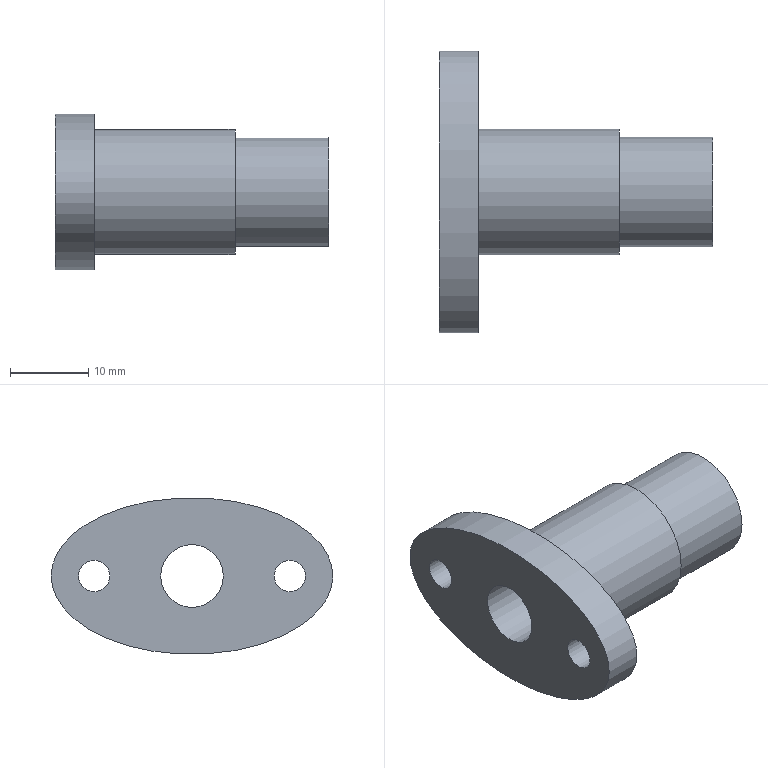Part | STEP file | 1-56.14 | 1 solid | 11 faces | box 35 x 36 x 20 mm | volume 6413 mm3 | cylinder 6 | plane 4 | spline 1 | commonest cylinder face diameters 4 x2 8 x2 14 x1 16 x1
STEP:
#1=CARTESIAN_POINT('',(0.,0.,0.));
#2=DIRECTION('',(0.,0.,1.));
#3=DIRECTION('',(1.,0.,0.));
#4=AXIS2_PLACEMENT_3D('',#1,#2,#3);
#5=CARTESIAN_POINT('',(-5.,18.,0.));
#6=VERTEX_POINT('',#5);
#7=CARTESIAN_POINT('',(-5.,0.,0.));
#8=DIRECTION('',(1.,0.,0.));
#9=DIRECTION('',(0.,1.,0.));
#10=AXIS2_PLACEMENT_3D('',#7,#8,#9);
#11=ELLIPSE('',#10,18.,10.);
#12=CARTESIAN_POINT('',(-5.,0.,-8.));
#13=DIRECTION('',(1.,0.,0.));
#14=DIRECTION('',(0.,0.,-1.));
#15=AXIS2_PLACEMENT_3D('',#12,#13,#14);
#16=PLANE('',#15);
#17=CARTESIAN_POINT('',(-8.,0.));
#18=DIRECTION('',(0.,1.));
#19=AXIS2_PLACEMENT_2D('',#17,#18);
#20=ELLIPSE('',#19,18.,10.);
#21=(GEOMETRIC_REPRESENTATION_CONTEXT(2)PARAMETRIC_REPRESENTATION_CONTEXT()REPRESENTATION_CONTEXT('',''));
#22=DEFINITIONAL_REPRESENTATION('',(#20),#21);
#23=PCURVE('',#16,#22);
#24=CARTESIAN_POINT('',(0.,18.,0.));
#25=CARTESIAN_POINT('',(-5.,18.,0.));
#26=CARTESIAN_POINT('',(0.,18.,10.));
#27=CARTESIAN_POINT('',(-5.,18.,10.));
#28=CARTESIAN_POINT('',(0.,0.,10.));
#29=CARTESIAN_POINT('',(-5.,0.,10.));
#30=CARTESIAN_POINT('',(0.,-18.,10.));
#31=CARTESIAN_POINT('',(-5.,-18.,10.));
#32=CARTESIAN_POINT('',(0.,-18.,0.));
#33=CARTESIAN_POINT('',(-5.,-18.,0.));
#34=CARTESIAN_POINT('',(0.,-18.,-10.));
#35=CARTESIAN_POINT('',(-5.,-18.,-10.));
#36=CARTESIAN_POINT('',(0.,0.,-10.));
#37=CARTESIAN_POINT('',(-5.,0.,-10.));
#38=CARTESIAN_POINT('',(0.,18.,-10.));
#39=CARTESIAN_POINT('',(-5.,18.,-10.));
#40=CARTESIAN_POINT('',(0.,18.,0.));
#41=CARTESIAN_POINT('',(-5.,18.,0.));
#42=(BOUNDED_SURFACE()B_SPLINE_SURFACE(2,1,((#24,#25),(#26,#27),(#28,#29),(#30,#31),(#32,#33),(#34,#35),(#36,#37),(#38,#39),(#40,#41)),.UNSPECIFIED.,.T.,.F.,.F.)B_SPLINE_SURFACE_WITH_KNOTS((1,2,2,2,2,2,1),(2,2),(-0.25,0.,0.25,0.5,0.75,1.,1.25),(0.,1.),.UNSPECIFIED.)GEOMETRIC_REPRESENTATION_ITEM()RATIONAL_B_SPLINE_SURFACE(((1.,1.),(0.7071,0.7071),(1.,1.),(0.7071,0.7071),(1.,1.),(0.7071,0.7071),(1.,1.),(0.7071,0.7071),(1.,1.)))REPRESENTATION_ITEM('')SURFACE());
#43=CARTESIAN_POINT('',(0.,1.));
#44=CARTESIAN_POINT('',(0.01678,1.));
#45=CARTESIAN_POINT('',(0.04854,1.));
#46=CARTESIAN_POINT('',(0.09277,1.));
#47=CARTESIAN_POINT('',(0.1357,1.));
#48=CARTESIAN_POINT('',(0.1791,1.));
#49=CARTESIAN_POINT('',(0.2245,1.));
#50=CARTESIAN_POINT('',(0.2755,1.));
#51=CARTESIAN_POINT('',(0.3209,1.));
#52=CARTESIAN_POINT('',(0.3643,1.));
#53=CARTESIAN_POINT('',(0.4073,1.));
#54=CARTESIAN_POINT('',(0.4512,1.));
#55=CARTESIAN_POINT('',(0.5,1.));
#56=CARTESIAN_POINT('',(0.5488,1.));
#57=CARTESIAN_POINT('',(0.5927,1.));
#58=CARTESIAN_POINT('',(0.6357,1.));
#59=CARTESIAN_POINT('',(0.6791,1.));
#60=CARTESIAN_POINT('',(0.7245,1.));
#61=CARTESIAN_POINT('',(0.7755,1.));
#62=CARTESIAN_POINT('',(0.8209,1.));
#63=CARTESIAN_POINT('',(0.8643,1.));
#64=CARTESIAN_POINT('',(0.9072,1.));
#65=CARTESIAN_POINT('',(0.9515,1.));
#66=CARTESIAN_POINT('',(0.9832,1.));
#67=CARTESIAN_POINT('',(1.,1.));
#68=B_SPLINE_CURVE_WITH_KNOTS('',3,(#43,#44,#45,#46,#47,#48,#49,#50,#51,#52,#53,#54,#55,#56,#57,#58,#59,#60,#61,#62,#63,#64,#65,#66,#67),.UNSPECIFIED.,.F.,.F.,(4,1,1,1,1,1,1,1,1,1,1,1,1,1,1,1,1,1,1,1,1,1,4),(0.,0.2856,0.5712,0.8568,1.142,1.428,1.714,1.999,2.285,2.57,2.856,3.142,3.427,3.713,3.998,4.284,4.57,4.855,5.141,5.426,5.712,5.998,6.283),.QUASI_UNIFORM_KNOTS.);
#69=(GEOMETRIC_REPRESENTATION_CONTEXT(2)PARAMETRIC_REPRESENTATION_CONTEXT()REPRESENTATION_CONTEXT('',''));
#70=DEFINITIONAL_REPRESENTATION('',(#68),#69);
#71=PCURVE('',#42,#70);
#72=SURFACE_CURVE('',#11,(#23,#71),.PCURVE_S1.);
#73=EDGE_CURVE('',#6,#6,#72,.T.);
#74=ORIENTED_EDGE('',*,*,#73,.T.);
#75=EDGE_LOOP('',(#74));
#76=FACE_BOUND('',#75,.F.);
#77=CARTESIAN_POINT('',(-5.,14.5,0.));
#78=VERTEX_POINT('',#77);
#79=CARTESIAN_POINT('',(-5.,12.5,0.));
#80=DIRECTION('',(-1.,0.,0.));
#81=DIRECTION('',(0.,1.,0.));
#82=AXIS2_PLACEMENT_3D('',#79,#80,#81);
#83=CIRCLE('',#82,2.);
#84=CARTESIAN_POINT('',(-8.,14.5));
#85=CARTESIAN_POINT('',(-4.536,14.5));
#86=CARTESIAN_POINT('',(-6.268,11.5));
#87=CARTESIAN_POINT('',(-8.,8.5));
#88=CARTESIAN_POINT('',(-9.732,11.5));
#89=CARTESIAN_POINT('',(-11.464,14.5));
#90=CARTESIAN_POINT('',(-8.,14.5));
#91=(BOUNDED_CURVE()B_SPLINE_CURVE(2,(#84,#85,#86,#87,#88,#89,#90),.UNSPECIFIED.,.T.,.F.)B_SPLINE_CURVE_WITH_KNOTS((1,2,2,2,2,1),(-2.094,0.,2.094,4.189,6.283,8.378),.UNSPECIFIED.)CURVE()GEOMETRIC_REPRESENTATION_ITEM()RATIONAL_B_SPLINE_CURVE((1.,0.5,1.,0.5,1.,0.5,1.))REPRESENTATION_ITEM(''));
#92=(GEOMETRIC_REPRESENTATION_CONTEXT(2)PARAMETRIC_REPRESENTATION_CONTEXT()REPRESENTATION_CONTEXT('',''));
#93=DEFINITIONAL_REPRESENTATION('',(#91),#92);
#94=PCURVE('',#16,#93);
#95=CARTESIAN_POINT('',(0.,12.5,0.));
#96=DIRECTION('',(-1.,0.,0.));
#97=DIRECTION('',(0.,1.,0.));
#98=AXIS2_PLACEMENT_3D('',#95,#96,#97);
#99=CYLINDRICAL_SURFACE('',#98,2.);
#100=CARTESIAN_POINT('',(0.,5.));
#101=DIRECTION('',(1.,0.));
#102=VECTOR('',#101,1.);
#103=LINE('',#100,#102);
#104=(GEOMETRIC_REPRESENTATION_CONTEXT(2)PARAMETRIC_REPRESENTATION_CONTEXT()REPRESENTATION_CONTEXT('',''));
#105=DEFINITIONAL_REPRESENTATION('',(#103),#104);
#106=PCURVE('',#99,#105);
#107=SURFACE_CURVE('',#83,(#94,#106),.PCURVE_S1.);
#108=EDGE_CURVE('',#78,#78,#107,.T.);
#109=ORIENTED_EDGE('',*,*,#108,.T.);
#110=EDGE_LOOP('',(#109));
#111=FACE_BOUND('',#110,.F.);
#112=CARTESIAN_POINT('',(-5.,-10.5,0.));
#113=VERTEX_POINT('',#112);
#114=CARTESIAN_POINT('',(-5.,-12.5,0.));
#115=DIRECTION('',(-1.,0.,0.));
#116=DIRECTION('',(0.,1.,0.));
#117=AXIS2_PLACEMENT_3D('',#114,#115,#116);
#118=CIRCLE('',#117,2.);
#119=CARTESIAN_POINT('',(-8.,-10.5));
#120=CARTESIAN_POINT('',(-4.536,-10.5));
#121=CARTESIAN_POINT('',(-6.268,-13.5));
#122=CARTESIAN_POINT('',(-8.,-16.5));
#123=CARTESIAN_POINT('',(-9.732,-13.5));
#124=CARTESIAN_POINT('',(-11.464,-10.5));
#125=CARTESIAN_POINT('',(-8.,-10.5));
#126=(BOUNDED_CURVE()B_SPLINE_CURVE(2,(#119,#120,#121,#122,#123,#124,#125),.UNSPECIFIED.,.T.,.F.)B_SPLINE_CURVE_WITH_KNOTS((1,2,2,2,2,1),(-2.094,0.,2.094,4.189,6.283,8.378),.UNSPECIFIED.)CURVE()GEOMETRIC_REPRESENTATION_ITEM()RATIONAL_B_SPLINE_CURVE((1.,0.5,1.,0.5,1.,0.5,1.))REPRESENTATION_ITEM(''));
#127=(GEOMETRIC_REPRESENTATION_CONTEXT(2)PARAMETRIC_REPRESENTATION_CONTEXT()REPRESENTATION_CONTEXT('',''));
#128=DEFINITIONAL_REPRESENTATION('',(#126),#127);
#129=PCURVE('',#16,#128);
#130=CARTESIAN_POINT('',(0.,-12.5,0.));
#131=DIRECTION('',(-1.,0.,0.));
#132=DIRECTION('',(0.,1.,0.));
#133=AXIS2_PLACEMENT_3D('',#130,#131,#132);
#134=CYLINDRICAL_SURFACE('',#133,2.);
#135=CARTESIAN_POINT('',(0.,5.));
#136=DIRECTION('',(1.,0.));
#137=VECTOR('',#136,1.);
#138=LINE('',#135,#137);
#139=(GEOMETRIC_REPRESENTATION_CONTEXT(2)PARAMETRIC_REPRESENTATION_CONTEXT()REPRESENTATION_CONTEXT('',''));
#140=DEFINITIONAL_REPRESENTATION('',(#138),#139);
#141=PCURVE('',#134,#140);
#142=SURFACE_CURVE('',#118,(#129,#141),.PCURVE_S1.);
#143=EDGE_CURVE('',#113,#113,#142,.T.);
#144=ORIENTED_EDGE('',*,*,#143,.T.);
#145=EDGE_LOOP('',(#144));
#146=FACE_BOUND('',#145,.F.);
#147=CARTESIAN_POINT('',(-5.,4.,0.));
#148=VERTEX_POINT('',#147);
#149=CARTESIAN_POINT('',(-5.,0.,0.));
#150=DIRECTION('',(-1.,0.,0.));
#151=DIRECTION('',(0.,1.,0.));
#152=AXIS2_PLACEMENT_3D('',#149,#150,#151);
#153=CIRCLE('',#152,4.);
#154=CARTESIAN_POINT('',(-8.,4.));
#155=CARTESIAN_POINT('',(-1.072,4.));
#156=CARTESIAN_POINT('',(-4.536,-2.));
#157=CARTESIAN_POINT('',(-8.,-8.));
#158=CARTESIAN_POINT('',(-11.464,-2.));
#159=CARTESIAN_POINT('',(-14.928,4.));
#160=CARTESIAN_POINT('',(-8.,4.));
#161=(BOUNDED_CURVE()B_SPLINE_CURVE(2,(#154,#155,#156,#157,#158,#159,#160),.UNSPECIFIED.,.T.,.F.)B_SPLINE_CURVE_WITH_KNOTS((1,2,2,2,2,1),(-2.094,0.,2.094,4.189,6.283,8.378),.UNSPECIFIED.)CURVE()GEOMETRIC_REPRESENTATION_ITEM()RATIONAL_B_SPLINE_CURVE((1.,0.5,1.,0.5,1.,0.5,1.))REPRESENTATION_ITEM(''));
#162=(GEOMETRIC_REPRESENTATION_CONTEXT(2)PARAMETRIC_REPRESENTATION_CONTEXT()REPRESENTATION_CONTEXT('',''));
#163=DEFINITIONAL_REPRESENTATION('',(#161),#162);
#164=PCURVE('',#16,#163);
#165=CARTESIAN_POINT('',(30.,0.,0.));
#166=DIRECTION('',(-1.,0.,0.));
#167=DIRECTION('',(0.,1.,0.));
#168=AXIS2_PLACEMENT_3D('',#165,#166,#167);
#169=CYLINDRICAL_SURFACE('',#168,4.);
#170=CARTESIAN_POINT('',(0.,35.));
#171=DIRECTION('',(1.,0.));
#172=VECTOR('',#171,1.);
#173=LINE('',#170,#172);
#174=(GEOMETRIC_REPRESENTATION_CONTEXT(2)PARAMETRIC_REPRESENTATION_CONTEXT()REPRESENTATION_CONTEXT('',''));
#175=DEFINITIONAL_REPRESENTATION('',(#173),#174);
#176=PCURVE('',#169,#175);
#177=SURFACE_CURVE('',#153,(#164,#176),.PCURVE_S1.);
#178=EDGE_CURVE('',#148,#148,#177,.T.);
#179=ORIENTED_EDGE('',*,*,#178,.T.);
#180=EDGE_LOOP('',(#179));
#181=FACE_BOUND('',#180,.F.);
#182=ADVANCED_FACE('',(#76,#111,#146,#181),#16,.F.);
#183=CARTESIAN_POINT('',(0.,18.,0.));
#184=VERTEX_POINT('',#183);
#185=CARTESIAN_POINT('',(0.,0.,0.));
#186=DIRECTION('',(1.,0.,0.));
#187=DIRECTION('',(0.,1.,0.));
#188=AXIS2_PLACEMENT_3D('',#185,#186,#187);
#189=ELLIPSE('',#188,18.,10.);
#190=CARTESIAN_POINT('',(0.,0.));
#191=CARTESIAN_POINT('',(0.01678,0.));
#192=CARTESIAN_POINT('',(0.04854,0.));
#193=CARTESIAN_POINT('',(0.09277,0.));
#194=CARTESIAN_POINT('',(0.1357,0.));
#195=CARTESIAN_POINT('',(0.1791,0.));
#196=CARTESIAN_POINT('',(0.2245,0.));
#197=CARTESIAN_POINT('',(0.2755,0.));
#198=CARTESIAN_POINT('',(0.3209,0.));
#199=CARTESIAN_POINT('',(0.3643,0.));
#200=CARTESIAN_POINT('',(0.4073,0.));
#201=CARTESIAN_POINT('',(0.4512,0.));
#202=CARTESIAN_POINT('',(0.5,0.));
#203=CARTESIAN_POINT('',(0.5488,0.));
#204=CARTESIAN_POINT('',(0.5927,0.));
#205=CARTESIAN_POINT('',(0.6357,0.));
#206=CARTESIAN_POINT('',(0.6791,0.));
#207=CARTESIAN_POINT('',(0.7245,0.));
#208=CARTESIAN_POINT('',(0.7755,0.));
#209=CARTESIAN_POINT('',(0.8209,0.));
#210=CARTESIAN_POINT('',(0.8643,0.));
#211=CARTESIAN_POINT('',(0.9072,0.));
#212=CARTESIAN_POINT('',(0.9515,0.));
#213=CARTESIAN_POINT('',(0.9832,0.));
#214=CARTESIAN_POINT('',(1.,0.));
#215=B_SPLINE_CURVE_WITH_KNOTS('',3,(#190,#191,#192,#193,#194,#195,#196,#197,#198,#199,#200,#201,#202,#203,#204,#205,#206,#207,#208,#209,#210,#211,#212,#213,#214),.UNSPECIFIED.,.F.,.F.,(4,1,1,1,1,1,1,1,1,1,1,1,1,1,1,1,1,1,1,1,1,1,4),(0.,0.2856,0.5712,0.8568,1.142,1.428,1.714,1.999,2.285,2.57,2.856,3.142,3.427,3.713,3.998,4.284,4.57,4.855,5.141,5.426,5.712,5.998,6.283),.QUASI_UNIFORM_KNOTS.);
#216=(GEOMETRIC_REPRESENTATION_CONTEXT(2)PARAMETRIC_REPRESENTATION_CONTEXT()REPRESENTATION_CONTEXT('',''));
#217=DEFINITIONAL_REPRESENTATION('',(#215),#216);
#218=PCURVE('',#42,#217);
#219=CARTESIAN_POINT('',(0.,0.,-8.));
#220=DIRECTION('',(1.,0.,0.));
#221=DIRECTION('',(0.,0.,-1.));
#222=AXIS2_PLACEMENT_3D('',#219,#220,#221);
#223=PLANE('',#222);
#224=CARTESIAN_POINT('',(-8.,0.));
#225=DIRECTION('',(0.,1.));
#226=AXIS2_PLACEMENT_2D('',#224,#225);
#227=ELLIPSE('',#226,18.,10.);
#228=(GEOMETRIC_REPRESENTATION_CONTEXT(2)PARAMETRIC_REPRESENTATION_CONTEXT()REPRESENTATION_CONTEXT('',''));
#229=DEFINITIONAL_REPRESENTATION('',(#227),#228);
#230=PCURVE('',#223,#229);
#231=SURFACE_CURVE('',#189,(#218,#230),.PCURVE_S1.);
#232=EDGE_CURVE('',#184,#184,#231,.T.);
#233=ORIENTED_EDGE('',*,*,#232,.T.);
#234=CARTESIAN_POINT('',(0.,18.,0.));
#235=DIRECTION('',(-1.,0.,0.));
#236=VECTOR('',#235,1.);
#237=LINE('',#234,#236);
#238=CARTESIAN_POINT('',(1.,0.));
#239=CARTESIAN_POINT('',(1.,1.));
#240=B_SPLINE_CURVE_WITH_KNOTS('',1,(#238,#239),.UNSPECIFIED.,.F.,.F.,(2,2),(0.,5.),.PIECEWISE_BEZIER_KNOTS.);
#241=(GEOMETRIC_REPRESENTATION_CONTEXT(2)PARAMETRIC_REPRESENTATION_CONTEXT()REPRESENTATION_CONTEXT('',''));
#242=DEFINITIONAL_REPRESENTATION('',(#240),#241);
#243=PCURVE('',#42,#242);
#244=CARTESIAN_POINT('',(0.,0.));
#245=CARTESIAN_POINT('',(0.,1.));
#246=B_SPLINE_CURVE_WITH_KNOTS('',1,(#244,#245),.UNSPECIFIED.,.F.,.F.,(2,2),(0.,5.),.PIECEWISE_BEZIER_KNOTS.);
#247=(GEOMETRIC_REPRESENTATION_CONTEXT(2)PARAMETRIC_REPRESENTATION_CONTEXT()REPRESENTATION_CONTEXT('',''));
#248=DEFINITIONAL_REPRESENTATION('',(#246),#247);
#249=PCURVE('',#42,#248);
#250=SEAM_CURVE('',#237,(#243,#249),.PCURVE_S1.);
#251=EDGE_CURVE('',#184,#6,#250,.T.);
#252=ORIENTED_EDGE('',*,*,#251,.T.);
#253=ORIENTED_EDGE('',*,*,#73,.F.);
#254=ORIENTED_EDGE('',*,*,#251,.F.);
#255=EDGE_LOOP('',(#233,#252,#253,#254));
#256=FACE_BOUND('',#255,.F.);
#257=ADVANCED_FACE('',(#256),#42,.F.);
#258=CARTESIAN_POINT('',(0.,14.5,0.));
#259=VERTEX_POINT('',#258);
#260=CARTESIAN_POINT('',(0.,12.5,0.));
#261=DIRECTION('',(-1.,0.,0.));
#262=DIRECTION('',(0.,1.,0.));
#263=AXIS2_PLACEMENT_3D('',#260,#261,#262);
#264=CIRCLE('',#263,2.);
#265=CARTESIAN_POINT('',(0.,0.));
#266=DIRECTION('',(1.,0.));
#267=VECTOR('',#266,1.);
#268=LINE('',#265,#267);
#269=(GEOMETRIC_REPRESENTATION_CONTEXT(2)PARAMETRIC_REPRESENTATION_CONTEXT()REPRESENTATION_CONTEXT('',''));
#270=DEFINITIONAL_REPRESENTATION('',(#268),#269);
#271=PCURVE('',#99,#270);
#272=CARTESIAN_POINT('',(-8.,14.5));
#273=CARTESIAN_POINT('',(-4.536,14.5));
#274=CARTESIAN_POINT('',(-6.268,11.5));
#275=CARTESIAN_POINT('',(-8.,8.5));
#276=CARTESIAN_POINT('',(-9.732,11.5));
#277=CARTESIAN_POINT('',(-11.464,14.5));
#278=CARTESIAN_POINT('',(-8.,14.5));
#279=(BOUNDED_CURVE()B_SPLINE_CURVE(2,(#272,#273,#274,#275,#276,#277,#278),.UNSPECIFIED.,.T.,.F.)B_SPLINE_CURVE_WITH_KNOTS((1,2,2,2,2,1),(-2.094,0.,2.094,4.189,6.283,8.378),.UNSPECIFIED.)CURVE()GEOMETRIC_REPRESENTATION_ITEM()RATIONAL_B_SPLINE_CURVE((1.,0.5,1.,0.5,1.,0.5,1.))REPRESENTATION_ITEM(''));
#280=(GEOMETRIC_REPRESENTATION_CONTEXT(2)PARAMETRIC_REPRESENTATION_CONTEXT()REPRESENTATION_CONTEXT('',''));
#281=DEFINITIONAL_REPRESENTATION('',(#279),#280);
#282=PCURVE('',#223,#281);
#283=SURFACE_CURVE('',#264,(#271,#282),.PCURVE_S1.);
#284=EDGE_CURVE('',#259,#259,#283,.T.);
#285=ORIENTED_EDGE('',*,*,#284,.T.);
#286=CARTESIAN_POINT('',(0.,14.5,0.));
#287=DIRECTION('',(-1.,0.,0.));
#288=VECTOR('',#287,1.);
#289=LINE('',#286,#288);
#290=CARTESIAN_POINT('',(6.283,0.));
#291=DIRECTION('',(0.,1.));
#292=VECTOR('',#291,1.);
#293=LINE('',#290,#292);
#294=(GEOMETRIC_REPRESENTATION_CONTEXT(2)PARAMETRIC_REPRESENTATION_CONTEXT()REPRESENTATION_CONTEXT('',''));
#295=DEFINITIONAL_REPRESENTATION('',(#293),#294);
#296=PCURVE('',#99,#295);
#297=CARTESIAN_POINT('',(0.,0.));
#298=DIRECTION('',(0.,1.));
#299=VECTOR('',#298,1.);
#300=LINE('',#297,#299);
#301=(GEOMETRIC_REPRESENTATION_CONTEXT(2)PARAMETRIC_REPRESENTATION_CONTEXT()REPRESENTATION_CONTEXT('',''));
#302=DEFINITIONAL_REPRESENTATION('',(#300),#301);
#303=PCURVE('',#99,#302);
#304=SEAM_CURVE('',#289,(#296,#303),.PCURVE_S1.);
#305=EDGE_CURVE('',#259,#78,#304,.T.);
#306=ORIENTED_EDGE('',*,*,#305,.T.);
#307=ORIENTED_EDGE('',*,*,#108,.F.);
#308=ORIENTED_EDGE('',*,*,#305,.F.);
#309=EDGE_LOOP('',(#285,#306,#307,#308));
#310=FACE_BOUND('',#309,.F.);
#311=ADVANCED_FACE('',(#310),#99,.F.);
#312=CARTESIAN_POINT('',(0.,-10.5,0.));
#313=VERTEX_POINT('',#312);
#314=CARTESIAN_POINT('',(0.,-12.5,0.));
#315=DIRECTION('',(-1.,0.,0.));
#316=DIRECTION('',(0.,1.,0.));
#317=AXIS2_PLACEMENT_3D('',#314,#315,#316);
#318=CIRCLE('',#317,2.);
#319=CARTESIAN_POINT('',(0.,0.));
#320=DIRECTION('',(1.,0.));
#321=VECTOR('',#320,1.);
#322=LINE('',#319,#321);
#323=(GEOMETRIC_REPRESENTATION_CONTEXT(2)PARAMETRIC_REPRESENTATION_CONTEXT()REPRESENTATION_CONTEXT('',''));
#324=DEFINITIONAL_REPRESENTATION('',(#322),#323);
#325=PCURVE('',#134,#324);
#326=CARTESIAN_POINT('',(-8.,-10.5));
#327=CARTESIAN_POINT('',(-4.536,-10.5));
#328=CARTESIAN_POINT('',(-6.268,-13.5));
#329=CARTESIAN_POINT('',(-8.,-16.5));
#330=CARTESIAN_POINT('',(-9.732,-13.5));
#331=CARTESIAN_POINT('',(-11.464,-10.5));
#332=CARTESIAN_POINT('',(-8.,-10.5));
#333=(BOUNDED_CURVE()B_SPLINE_CURVE(2,(#326,#327,#328,#329,#330,#331,#332),.UNSPECIFIED.,.T.,.F.)B_SPLINE_CURVE_WITH_KNOTS((1,2,2,2,2,1),(-2.094,0.,2.094,4.189,6.283,8.378),.UNSPECIFIED.)CURVE()GEOMETRIC_REPRESENTATION_ITEM()RATIONAL_B_SPLINE_CURVE((1.,0.5,1.,0.5,1.,0.5,1.))REPRESENTATION_ITEM(''));
#334=(GEOMETRIC_REPRESENTATION_CONTEXT(2)PARAMETRIC_REPRESENTATION_CONTEXT()REPRESENTATION_CONTEXT('',''));
#335=DEFINITIONAL_REPRESENTATION('',(#333),#334);
#336=PCURVE('',#223,#335);
#337=SURFACE_CURVE('',#318,(#325,#336),.PCURVE_S1.);
#338=EDGE_CURVE('',#313,#313,#337,.T.);
#339=ORIENTED_EDGE('',*,*,#338,.T.);
#340=CARTESIAN_POINT('',(0.,-10.5,0.));
#341=DIRECTION('',(-1.,0.,0.));
#342=VECTOR('',#341,1.);
#343=LINE('',#340,#342);
#344=CARTESIAN_POINT('',(6.283,0.));
#345=DIRECTION('',(0.,1.));
#346=VECTOR('',#345,1.);
#347=LINE('',#344,#346);
#348=(GEOMETRIC_REPRESENTATION_CONTEXT(2)PARAMETRIC_REPRESENTATION_CONTEXT()REPRESENTATION_CONTEXT('',''));
#349=DEFINITIONAL_REPRESENTATION('',(#347),#348);
#350=PCURVE('',#134,#349);
#351=CARTESIAN_POINT('',(0.,0.));
#352=DIRECTION('',(0.,1.));
#353=VECTOR('',#352,1.);
#354=LINE('',#351,#353);
#355=(GEOMETRIC_REPRESENTATION_CONTEXT(2)PARAMETRIC_REPRESENTATION_CONTEXT()REPRESENTATION_CONTEXT('',''));
#356=DEFINITIONAL_REPRESENTATION('',(#354),#355);
#357=PCURVE('',#134,#356);
#358=SEAM_CURVE('',#343,(#350,#357),.PCURVE_S1.);
#359=EDGE_CURVE('',#313,#113,#358,.T.);
#360=ORIENTED_EDGE('',*,*,#359,.T.);
#361=ORIENTED_EDGE('',*,*,#143,.F.);
#362=ORIENTED_EDGE('',*,*,#359,.F.);
#363=EDGE_LOOP('',(#339,#360,#361,#362));
#364=FACE_BOUND('',#363,.F.);
#365=ADVANCED_FACE('',(#364),#134,.F.);
#366=ORIENTED_EDGE('',*,*,#232,.T.);
#367=EDGE_LOOP('',(#366));
#368=FACE_BOUND('',#367,.T.);
#369=CARTESIAN_POINT('',(0.,8.,0.));
#370=VERTEX_POINT('',#369);
#371=CARTESIAN_POINT('',(0.,0.,0.));
#372=DIRECTION('',(1.,0.,0.));
#373=DIRECTION('',(0.,1.,0.));
#374=AXIS2_PLACEMENT_3D('',#371,#372,#373);
#375=CIRCLE('',#374,8.);
#376=CARTESIAN_POINT('',(-8.,0.));
#377=DIRECTION('',(0.,1.));
#378=AXIS2_PLACEMENT_2D('',#376,#377);
#379=CIRCLE('',#378,8.);
#380=(GEOMETRIC_REPRESENTATION_CONTEXT(2)PARAMETRIC_REPRESENTATION_CONTEXT()REPRESENTATION_CONTEXT('',''));
#381=DEFINITIONAL_REPRESENTATION('',(#379),#380);
#382=PCURVE('',#223,#381);
#383=CARTESIAN_POINT('',(0.,0.,0.));
#384=DIRECTION('',(1.,0.,0.));
#385=DIRECTION('',(0.,1.,0.));
#386=AXIS2_PLACEMENT_3D('',#383,#384,#385);
#387=CYLINDRICAL_SURFACE('',#386,8.);
#388=CARTESIAN_POINT('',(0.,0.));
#389=DIRECTION('',(1.,0.));
#390=VECTOR('',#389,1.);
#391=LINE('',#388,#390);
#392=(GEOMETRIC_REPRESENTATION_CONTEXT(2)PARAMETRIC_REPRESENTATION_CONTEXT()REPRESENTATION_CONTEXT('',''));
#393=DEFINITIONAL_REPRESENTATION('',(#391),#392);
#394=PCURVE('',#387,#393);
#395=SURFACE_CURVE('',#375,(#382,#394),.PCURVE_S1.);
#396=EDGE_CURVE('',#370,#370,#395,.T.);
#397=ORIENTED_EDGE('',*,*,#396,.F.);
#398=EDGE_LOOP('',(#397));
#399=FACE_BOUND('',#398,.T.);
#400=ORIENTED_EDGE('',*,*,#284,.T.);
#401=EDGE_LOOP('',(#400));
#402=FACE_BOUND('',#401,.T.);
#403=ORIENTED_EDGE('',*,*,#338,.T.);
#404=EDGE_LOOP('',(#403));
#405=FACE_BOUND('',#404,.T.);
#406=ADVANCED_FACE('',(#368,#399,#402,#405),#223,.T.);
#407=ORIENTED_EDGE('',*,*,#396,.T.);
#408=CARTESIAN_POINT('',(18.,8.,0.));
#409=VERTEX_POINT('',#408);
#410=CARTESIAN_POINT('',(0.,8.,0.));
#411=DIRECTION('',(1.,0.,0.));
#412=VECTOR('',#411,1.);
#413=LINE('',#410,#412);
#414=CARTESIAN_POINT('',(6.283,0.));
#415=DIRECTION('',(0.,1.));
#416=VECTOR('',#415,1.);
#417=LINE('',#414,#416);
#418=(GEOMETRIC_REPRESENTATION_CONTEXT(2)PARAMETRIC_REPRESENTATION_CONTEXT()REPRESENTATION_CONTEXT('',''));
#419=DEFINITIONAL_REPRESENTATION('',(#417),#418);
#420=PCURVE('',#387,#419);
#421=CARTESIAN_POINT('',(0.,0.));
#422=DIRECTION('',(0.,1.));
#423=VECTOR('',#422,1.);
#424=LINE('',#421,#423);
#425=(GEOMETRIC_REPRESENTATION_CONTEXT(2)PARAMETRIC_REPRESENTATION_CONTEXT()REPRESENTATION_CONTEXT('',''));
#426=DEFINITIONAL_REPRESENTATION('',(#424),#425);
#427=PCURVE('',#387,#426);
#428=SEAM_CURVE('',#413,(#420,#427),.PCURVE_S1.);
#429=EDGE_CURVE('',#370,#409,#428,.T.);
#430=ORIENTED_EDGE('',*,*,#429,.T.);
#431=CARTESIAN_POINT('',(18.,0.,0.));
#432=DIRECTION('',(1.,0.,0.));
#433=DIRECTION('',(0.,1.,0.));
#434=AXIS2_PLACEMENT_3D('',#431,#432,#433);
#435=CIRCLE('',#434,8.);
#436=CARTESIAN_POINT('',(0.,18.));
#437=DIRECTION('',(1.,0.));
#438=VECTOR('',#437,1.);
#439=LINE('',#436,#438);
#440=(GEOMETRIC_REPRESENTATION_CONTEXT(2)PARAMETRIC_REPRESENTATION_CONTEXT()REPRESENTATION_CONTEXT('',''));
#441=DEFINITIONAL_REPRESENTATION('',(#439),#440);
#442=PCURVE('',#387,#441);
#443=CARTESIAN_POINT('',(18.,-2.144,0.));
#444=DIRECTION('',(1.,0.,0.));
#445=DIRECTION('',(0.,0.,-1.));
#446=AXIS2_PLACEMENT_3D('',#443,#444,#445);
#447=PLANE('',#446);
#448=CARTESIAN_POINT('',(0.,2.144));
#449=DIRECTION('',(0.,1.));
#450=AXIS2_PLACEMENT_2D('',#448,#449);
#451=CIRCLE('',#450,8.);
#452=(GEOMETRIC_REPRESENTATION_CONTEXT(2)PARAMETRIC_REPRESENTATION_CONTEXT()REPRESENTATION_CONTEXT('',''));
#453=DEFINITIONAL_REPRESENTATION('',(#451),#452);
#454=PCURVE('',#447,#453);
#455=SURFACE_CURVE('',#435,(#442,#454),.PCURVE_S1.);
#456=EDGE_CURVE('',#409,#409,#455,.T.);
#457=ORIENTED_EDGE('',*,*,#456,.F.);
#458=ORIENTED_EDGE('',*,*,#429,.F.);
#459=EDGE_LOOP('',(#407,#430,#457,#458));
#460=FACE_BOUND('',#459,.T.);
#461=ADVANCED_FACE('',(#460),#387,.T.);
#462=ORIENTED_EDGE('',*,*,#456,.T.);
#463=EDGE_LOOP('',(#462));
#464=FACE_BOUND('',#463,.T.);
#465=CARTESIAN_POINT('',(18.,7.,0.));
#466=VERTEX_POINT('',#465);
#467=CARTESIAN_POINT('',(18.,0.,0.));
#468=DIRECTION('',(1.,0.,0.));
#469=DIRECTION('',(0.,1.,0.));
#470=AXIS2_PLACEMENT_3D('',#467,#468,#469);
#471=CIRCLE('',#470,7.);
#472=CARTESIAN_POINT('',(0.,2.144));
#473=DIRECTION('',(0.,1.));
#474=AXIS2_PLACEMENT_2D('',#472,#473);
#475=CIRCLE('',#474,7.);
#476=(GEOMETRIC_REPRESENTATION_CONTEXT(2)PARAMETRIC_REPRESENTATION_CONTEXT()REPRESENTATION_CONTEXT('',''));
#477=DEFINITIONAL_REPRESENTATION('',(#475),#476);
#478=PCURVE('',#447,#477);
#479=CARTESIAN_POINT('',(18.,0.,0.));
#480=DIRECTION('',(1.,0.,0.));
#481=DIRECTION('',(0.,1.,0.));
#482=AXIS2_PLACEMENT_3D('',#479,#480,#481);
#483=CYLINDRICAL_SURFACE('',#482,7.);
#484=CARTESIAN_POINT('',(0.,0.));
#485=DIRECTION('',(1.,0.));
#486=VECTOR('',#485,1.);
#487=LINE('',#484,#486);
#488=(GEOMETRIC_REPRESENTATION_CONTEXT(2)PARAMETRIC_REPRESENTATION_CONTEXT()REPRESENTATION_CONTEXT('',''));
#489=DEFINITIONAL_REPRESENTATION('',(#487),#488);
#490=PCURVE('',#483,#489);
#491=SURFACE_CURVE('',#471,(#478,#490),.PCURVE_S1.);
#492=EDGE_CURVE('',#466,#466,#491,.T.);
#493=ORIENTED_EDGE('',*,*,#492,.F.);
#494=EDGE_LOOP('',(#493));
#495=FACE_BOUND('',#494,.T.);
#496=ADVANCED_FACE('',(#464,#495),#447,.T.);
#497=CARTESIAN_POINT('',(30.,7.,0.));
#498=VERTEX_POINT('',#497);
#499=CARTESIAN_POINT('',(30.,0.,0.));
#500=DIRECTION('',(1.,0.,0.));
#501=DIRECTION('',(0.,1.,0.));
#502=AXIS2_PLACEMENT_3D('',#499,#500,#501);
#503=CIRCLE('',#502,7.);
#504=CARTESIAN_POINT('',(30.,-1.876,0.));
#505=DIRECTION('',(1.,0.,0.));
#506=DIRECTION('',(0.,0.,-1.));
#507=AXIS2_PLACEMENT_3D('',#504,#505,#506);
#508=PLANE('',#507);
#509=CARTESIAN_POINT('',(0.,1.876));
#510=DIRECTION('',(0.,1.));
#511=AXIS2_PLACEMENT_2D('',#509,#510);
#512=CIRCLE('',#511,7.);
#513=(GEOMETRIC_REPRESENTATION_CONTEXT(2)PARAMETRIC_REPRESENTATION_CONTEXT()REPRESENTATION_CONTEXT('',''));
#514=DEFINITIONAL_REPRESENTATION('',(#512),#513);
#515=PCURVE('',#508,#514);
#516=CARTESIAN_POINT('',(0.,12.));
#517=DIRECTION('',(1.,0.));
#518=VECTOR('',#517,1.);
#519=LINE('',#516,#518);
#520=(GEOMETRIC_REPRESENTATION_CONTEXT(2)PARAMETRIC_REPRESENTATION_CONTEXT()REPRESENTATION_CONTEXT('',''));
#521=DEFINITIONAL_REPRESENTATION('',(#519),#520);
#522=PCURVE('',#483,#521);
#523=SURFACE_CURVE('',#503,(#515,#522),.PCURVE_S1.);
#524=EDGE_CURVE('',#498,#498,#523,.T.);
#525=ORIENTED_EDGE('',*,*,#524,.T.);
#526=EDGE_LOOP('',(#525));
#527=FACE_BOUND('',#526,.T.);
#528=CARTESIAN_POINT('',(30.,4.,0.));
#529=VERTEX_POINT('',#528);
#530=CARTESIAN_POINT('',(30.,0.,0.));
#531=DIRECTION('',(-1.,0.,0.));
#532=DIRECTION('',(0.,1.,0.));
#533=AXIS2_PLACEMENT_3D('',#530,#531,#532);
#534=CIRCLE('',#533,4.);
#535=CARTESIAN_POINT('',(0.,5.876));
#536=CARTESIAN_POINT('',(6.928,5.876));
#537=CARTESIAN_POINT('',(3.464,-0.1244));
#538=CARTESIAN_POINT('',(0.,-6.124));
#539=CARTESIAN_POINT('',(-3.464,-0.1244));
#540=CARTESIAN_POINT('',(-6.928,5.876));
#541=CARTESIAN_POINT('',(0.,5.876));
#542=(BOUNDED_CURVE()B_SPLINE_CURVE(2,(#535,#536,#537,#538,#539,#540,#541),.UNSPECIFIED.,.T.,.F.)B_SPLINE_CURVE_WITH_KNOTS((1,2,2,2,2,1),(-2.094,0.,2.094,4.189,6.283,8.378),.UNSPECIFIED.)CURVE()GEOMETRIC_REPRESENTATION_ITEM()RATIONAL_B_SPLINE_CURVE((1.,0.5,1.,0.5,1.,0.5,1.))REPRESENTATION_ITEM(''));
#543=(GEOMETRIC_REPRESENTATION_CONTEXT(2)PARAMETRIC_REPRESENTATION_CONTEXT()REPRESENTATION_CONTEXT('',''));
#544=DEFINITIONAL_REPRESENTATION('',(#542),#543);
#545=PCURVE('',#508,#544);
#546=CARTESIAN_POINT('',(30.,0.,0.));
#547=DIRECTION('',(-1.,0.,0.));
#548=DIRECTION('',(0.,1.,0.));
#549=AXIS2_PLACEMENT_3D('',#546,#547,#548);
#550=CYLINDRICAL_SURFACE('',#549,4.);
#551=CARTESIAN_POINT('',(0.,0.));
#552=DIRECTION('',(1.,0.));
#553=VECTOR('',#552,1.);
#554=LINE('',#551,#553);
#555=(GEOMETRIC_REPRESENTATION_CONTEXT(2)PARAMETRIC_REPRESENTATION_CONTEXT()REPRESENTATION_CONTEXT('',''));
#556=DEFINITIONAL_REPRESENTATION('',(#554),#555);
#557=PCURVE('',#550,#556);
#558=SURFACE_CURVE('',#534,(#545,#557),.PCURVE_S1.);
#559=EDGE_CURVE('',#529,#529,#558,.T.);
#560=ORIENTED_EDGE('',*,*,#559,.T.);
#561=EDGE_LOOP('',(#560));
#562=FACE_BOUND('',#561,.T.);
#563=ADVANCED_FACE('',(#527,#562),#508,.T.);
#564=ORIENTED_EDGE('',*,*,#492,.T.);
#565=CARTESIAN_POINT('',(18.,7.,0.));
#566=DIRECTION('',(1.,0.,0.));
#567=VECTOR('',#566,1.);
#568=LINE('',#565,#567);
#569=CARTESIAN_POINT('',(6.283,0.));
#570=DIRECTION('',(0.,1.));
#571=VECTOR('',#570,1.);
#572=LINE('',#569,#571);
#573=(GEOMETRIC_REPRESENTATION_CONTEXT(2)PARAMETRIC_REPRESENTATION_CONTEXT()REPRESENTATION_CONTEXT('',''));
#574=DEFINITIONAL_REPRESENTATION('',(#572),#573);
#575=PCURVE('',#483,#574);
#576=CARTESIAN_POINT('',(0.,0.));
#577=DIRECTION('',(0.,1.));
#578=VECTOR('',#577,1.);
#579=LINE('',#576,#578);
#580=(GEOMETRIC_REPRESENTATION_CONTEXT(2)PARAMETRIC_REPRESENTATION_CONTEXT()REPRESENTATION_CONTEXT('',''));
#581=DEFINITIONAL_REPRESENTATION('',(#579),#580);
#582=PCURVE('',#483,#581);
#583=SEAM_CURVE('',#568,(#575,#582),.PCURVE_S1.);
#584=EDGE_CURVE('',#466,#498,#583,.T.);
#585=ORIENTED_EDGE('',*,*,#584,.T.);
#586=ORIENTED_EDGE('',*,*,#524,.F.);
#587=ORIENTED_EDGE('',*,*,#584,.F.);
#588=EDGE_LOOP('',(#564,#585,#586,#587));
#589=FACE_BOUND('',#588,.T.);
#590=ADVANCED_FACE('',(#589),#483,.T.);
#591=ORIENTED_EDGE('',*,*,#559,.T.);
#592=CARTESIAN_POINT('',(15.,4.,0.));
#593=VERTEX_POINT('',#592);
#594=CARTESIAN_POINT('',(15.,4.,0.));
#595=DIRECTION('',(1.,0.,0.));
#596=VECTOR('',#595,1.);
#597=LINE('',#594,#596);
#598=CARTESIAN_POINT('',(6.283,15.));
#599=DIRECTION('',(0.,-1.));
#600=VECTOR('',#599,1.);
#601=LINE('',#598,#600);
#602=(GEOMETRIC_REPRESENTATION_CONTEXT(2)PARAMETRIC_REPRESENTATION_CONTEXT()REPRESENTATION_CONTEXT('',''));
#603=DEFINITIONAL_REPRESENTATION('',(#601),#602);
#604=PCURVE('',#550,#603);
#605=CARTESIAN_POINT('',(0.,15.));
#606=DIRECTION('',(0.,-1.));
#607=VECTOR('',#606,1.);
#608=LINE('',#605,#607);
#609=(GEOMETRIC_REPRESENTATION_CONTEXT(2)PARAMETRIC_REPRESENTATION_CONTEXT()REPRESENTATION_CONTEXT('',''));
#610=DEFINITIONAL_REPRESENTATION('',(#608),#609);
#611=PCURVE('',#550,#610);
#612=SEAM_CURVE('',#597,(#604,#611),.PCURVE_S1.);
#613=EDGE_CURVE('',#593,#529,#612,.T.);
#614=ORIENTED_EDGE('',*,*,#613,.F.);
#615=CARTESIAN_POINT('',(15.,0.,0.));
#616=DIRECTION('',(-1.,0.,0.));
#617=DIRECTION('',(0.,1.,0.));
#618=AXIS2_PLACEMENT_3D('',#615,#616,#617);
#619=CIRCLE('',#618,4.);
#620=CARTESIAN_POINT('',(0.,15.));
#621=DIRECTION('',(1.,0.));
#622=VECTOR('',#621,1.);
#623=LINE('',#620,#622);
#624=(GEOMETRIC_REPRESENTATION_CONTEXT(2)PARAMETRIC_REPRESENTATION_CONTEXT()REPRESENTATION_CONTEXT('',''));
#625=DEFINITIONAL_REPRESENTATION('',(#623),#624);
#626=PCURVE('',#550,#625);
#627=CARTESIAN_POINT('',(0.,15.));
#628=DIRECTION('',(1.,0.));
#629=VECTOR('',#628,1.);
#630=LINE('',#627,#629);
#631=(GEOMETRIC_REPRESENTATION_CONTEXT(2)PARAMETRIC_REPRESENTATION_CONTEXT()REPRESENTATION_CONTEXT('',''));
#632=DEFINITIONAL_REPRESENTATION('',(#630),#631);
#633=PCURVE('',#169,#632);
#634=SURFACE_CURVE('',#619,(#626,#633),.PCURVE_S1.);
#635=EDGE_CURVE('',#593,#593,#634,.T.);
#636=ORIENTED_EDGE('',*,*,#635,.F.);
#637=ORIENTED_EDGE('',*,*,#613,.T.);
#638=EDGE_LOOP('',(#591,#614,#636,#637));
#639=FACE_BOUND('',#638,.F.);
#640=ADVANCED_FACE('',(#639),#550,.F.);
#641=ORIENTED_EDGE('',*,*,#178,.F.);
#642=CARTESIAN_POINT('',(-5.,4.,0.));
#643=DIRECTION('',(1.,0.,0.));
#644=VECTOR('',#643,1.);
#645=LINE('',#642,#644);
#646=CARTESIAN_POINT('',(0.,35.));
#647=DIRECTION('',(0.,-1.));
#648=VECTOR('',#647,1.);
#649=LINE('',#646,#648);
#650=(GEOMETRIC_REPRESENTATION_CONTEXT(2)PARAMETRIC_REPRESENTATION_CONTEXT()REPRESENTATION_CONTEXT('',''));
#651=DEFINITIONAL_REPRESENTATION('',(#649),#650);
#652=PCURVE('',#169,#651);
#653=CARTESIAN_POINT('',(6.283,35.));
#654=DIRECTION('',(0.,-1.));
#655=VECTOR('',#654,1.);
#656=LINE('',#653,#655);
#657=(GEOMETRIC_REPRESENTATION_CONTEXT(2)PARAMETRIC_REPRESENTATION_CONTEXT()REPRESENTATION_CONTEXT('',''));
#658=DEFINITIONAL_REPRESENTATION('',(#656),#657);
#659=PCURVE('',#169,#658);
#660=SEAM_CURVE('',#645,(#652,#659),.PCURVE_S1.);
#661=EDGE_CURVE('',#148,#593,#660,.T.);
#662=ORIENTED_EDGE('',*,*,#661,.T.);
#663=ORIENTED_EDGE('',*,*,#635,.T.);
#664=ORIENTED_EDGE('',*,*,#661,.F.);
#665=EDGE_LOOP('',(#641,#662,#663,#664));
#666=FACE_BOUND('',#665,.F.);
#667=ADVANCED_FACE('',(#666),#169,.F.);
#668=CLOSED_SHELL('',(#182,#257,#311,#365,#406,#461,#496,#563,#590,#640,#667));
#669=MANIFOLD_SOLID_BREP('',#668);
#670=(LENGTH_UNIT()NAMED_UNIT(*)SI_UNIT(.MILLI.,.METRE.));
#671=UNCERTAINTY_MEASURE_WITH_UNIT(LENGTH_MEASURE(0.0000001),#670,'','');
#672=(NAMED_UNIT(*)PLANE_ANGLE_UNIT()SI_UNIT($,.RADIAN.));
#673=(NAMED_UNIT(*)SI_UNIT($,.STERADIAN.)SOLID_ANGLE_UNIT());
#674=(GEOMETRIC_REPRESENTATION_CONTEXT(3)GLOBAL_UNCERTAINTY_ASSIGNED_CONTEXT((#671))GLOBAL_UNIT_ASSIGNED_CONTEXT((#670,#672,#673))REPRESENTATION_CONTEXT('',''));
#675=ADVANCED_BREP_SHAPE_REPRESENTATION('',(#4,#669),#674);